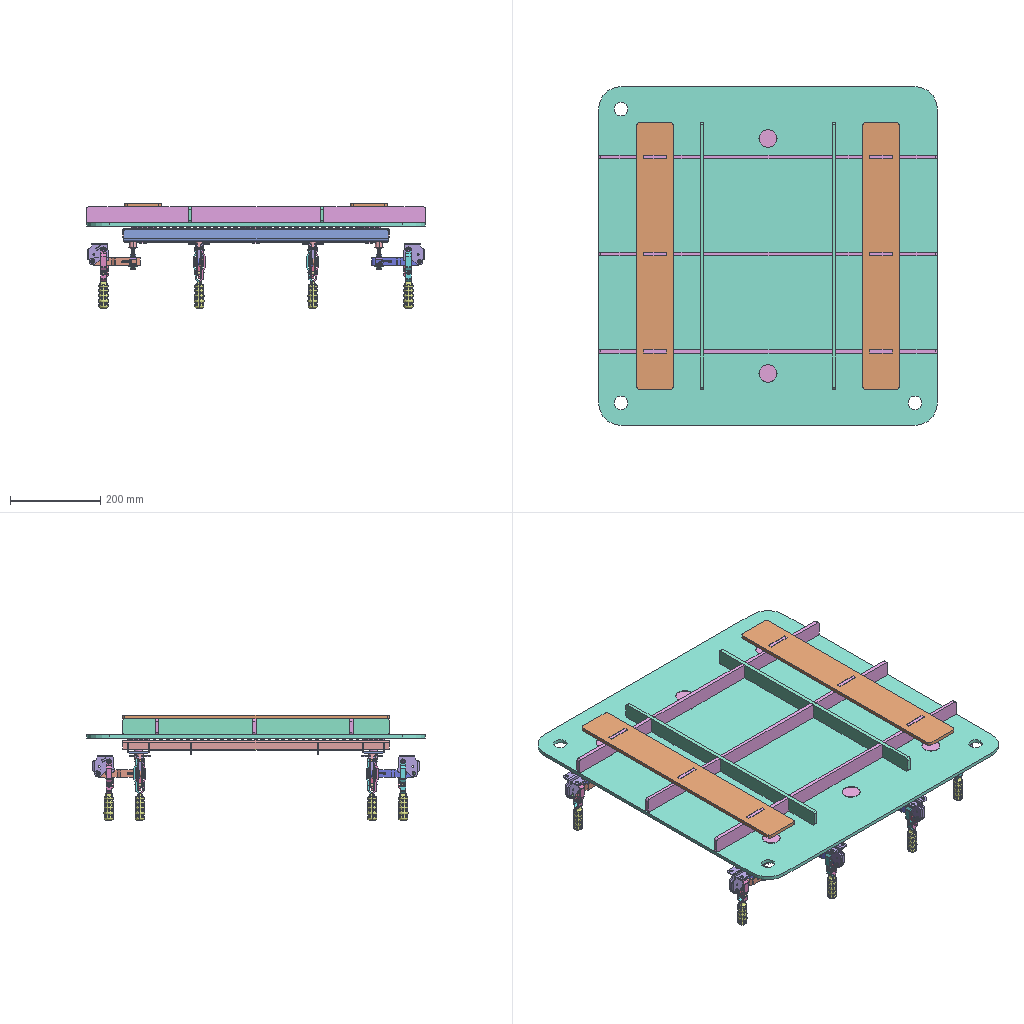Assembly | SolidWorks | 10 different items | 30 placed | box 750 x 750 x 234 mm
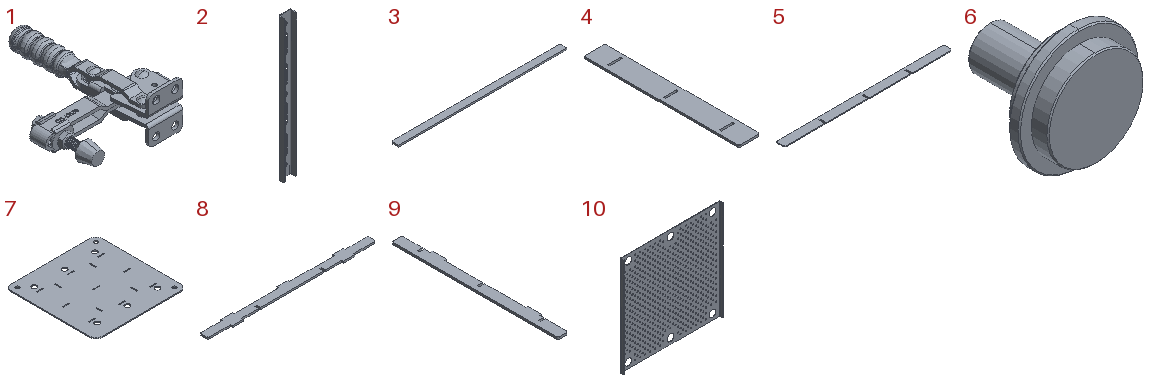Parts list (item | quantity | size | volume | features):
1 | x8 | 116.904 x 150.116 x 46 mm | 60512 mm3 | features BaseBody 18
2 | x2 | 50 x 26 x 585.4 mm | 111122 mm3 | features Chamfer 1, FlatPattern 1, ICE 1, SMBaseFlange 1, SheetMetal 1
3 | x3 | 470 x 20 x 4.5 mm | 42188 mm3 | features Chamfer 1, FlatPattern 1, SMBaseFlange 1, SheetMetal 1
4 | x2 | 80 x 590 x 8 mm | 367828 mm3 | features Fillet 1, FlatPattern 1, SMBaseFlange 1, SheetMetal 1
5 | x2 | 585.4 x 30 x 3 mm | 51728 mm3 | features FlatPattern 1, SMBaseFlange 1, SheetMetal 1
6 | x6 | 50 x 44.5 x 50 mm | 30963 mm3 | features Chamfer 1, Revolution 1
7 | x1 | 750 x 750 x 8 mm | 4363949 mm3 | features FlatPattern 1, ICE 1, SMBaseFlange 1, SheetMetal 1
8 | x3 | 750 x 49.5 x 8 mm | 222099 mm3 | features Fillet 2, FlatPattern 1, ICE 1, SMBaseFlange 1, SheetMetal 1
9 | x2 | 42.5 x 590 x 8 mm | 167562 mm3 | features Fillet 2, FlatPattern 1, ICE 1, SMBaseFlange 1, SheetMetal 1
10 | x1 | - | 887522 mm3 | features LPattern 6, FormToolInstance 4, MirrorPattern 2, FlatPattern 1, ICE 1, SMBaseFlange 1, SheetMetal 1
Mates (type | each side: item.copy, entity, surface, feature):
Coincident | 10.1 face plane Base-Flange1 | 2.1 face plane Base-Flange1 | 2 times
Concentric | 10.1 face cylinder Cut-Extrude1 | 2.1 face cylinder Cut-Extrude1
Coincident | 10.1 face plane Base-Flange1 | 3.1 face plane Base-Flange1
Coincident | 2.1 face plane Base-Flange1 | 3.1 face plane Base-Flange1
DistanceDim | 10.1 face plane Base-Flange1 | 3.1 face plane Base-Flange1
InPlace | 6.1 plane | assembly plane
InPlace | 6.2 face plane Revolve1 | 7.1 plane
Coincident | 2.1 face plane Base-Flange1 | 1.1 face plane
DistanceDim | 1.1 face plane | 2.1 face plane Base-Flange1
InPlace | 5.1 plane | assembly plane
InPlace | 8.1 plane | assembly plane
Coincident | 2.2 face plane Base-Flange1 | 1.2 face plane
InPlace | 9.1 plane | assembly plane
InPlace | 8.1 face plane Base-Flange1 | 4.1 plane